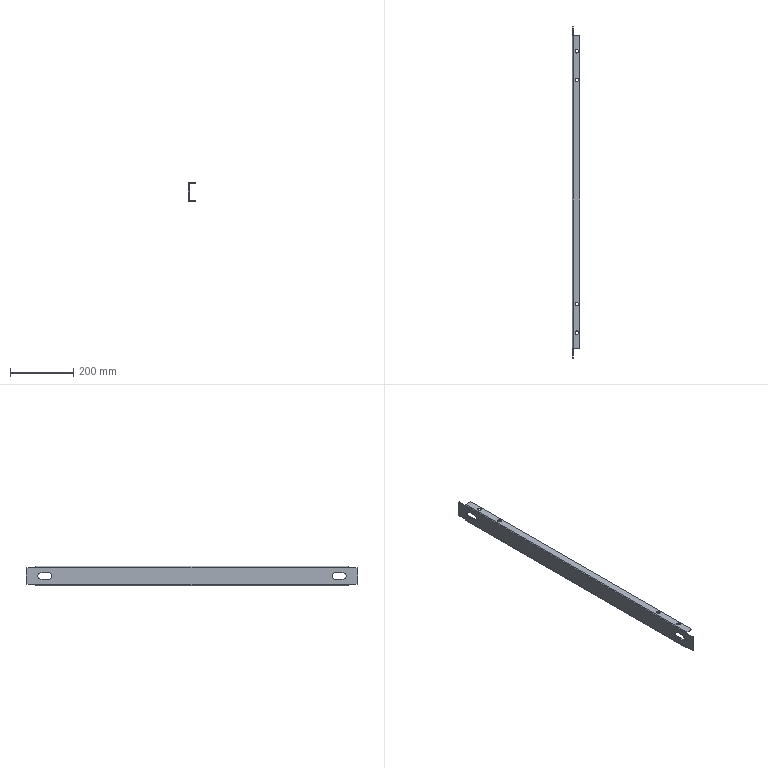Part | 1 solid | 58 faces | box 25 x 1053 x 62 mm | volume 313367 mm3 | plane 30 | cylinder 28 | commonest cylinder face diameters 11 x16 6 x4 20 x4 0.4 x2 6.4 x2